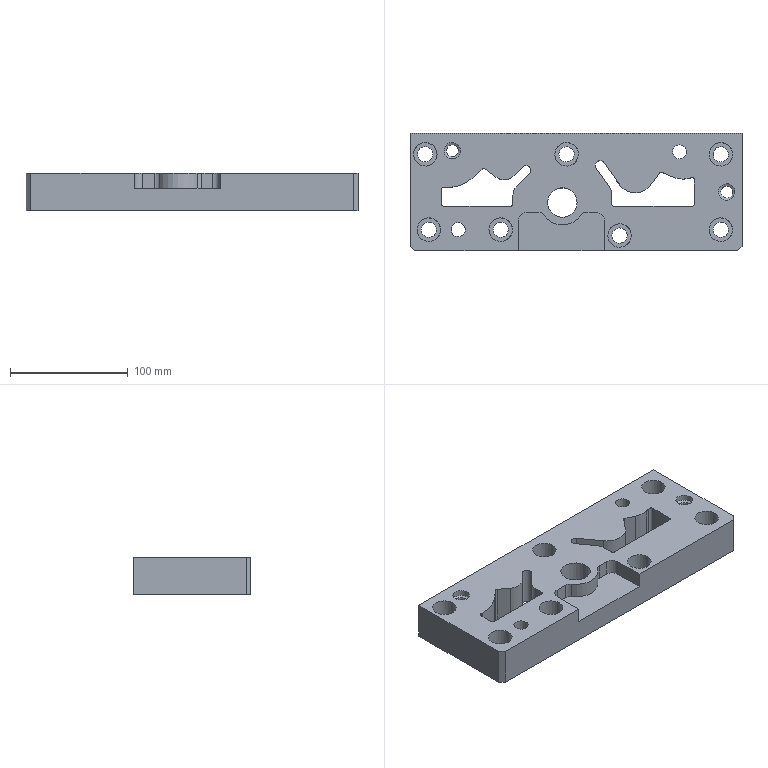Part | STEP file | gslz 2016.10.28-13_id170_x_t | 1 solid | 84 faces | box 282 x 100 x 32 mm | volume 692522 mm3 | cylinder 46 | plane 36 | cone 2 | commonest cylinder face diameters 4 x10 20 x9 13 x7 14 x4 8 x2 10 x2